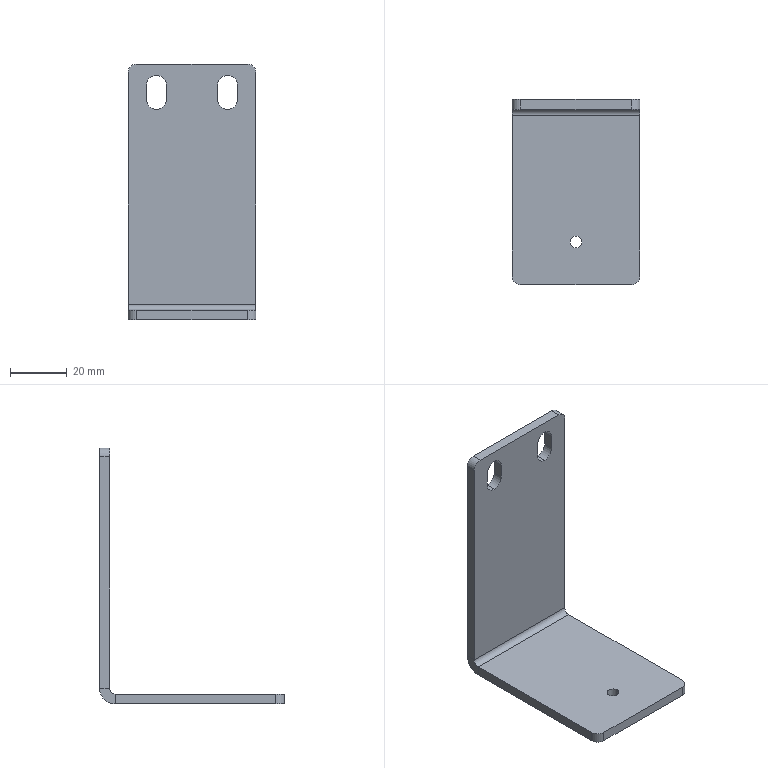Part | SolidWorks | features HoleWzd 2, EdgeFlange 1, Fillet 1, FlatPattern 1, ICE 1, MirrorPattern 1, SMBaseFlange 1, SheetMetal 1 | 1 solid | 30 faces | box 45 x 65 x 90 mm | volume 23018 mm3 | plane 16 | cylinder 14 | commonest cylinder face diameters 7 x6 6 x4 4.2 x2 4 x1 11 x1
STEP:
#1=CARTESIAN_POINT('',(16.,32.5,74.));
#2=VERTEX_POINT('',#1);
#3=CARTESIAN_POINT('',(12.5,32.5,70.5));
#4=VERTEX_POINT('',#3);
#5=CARTESIAN_POINT('',(12.5,32.5,74.));
#6=DIRECTION('',(0.,1.,0.));
#7=DIRECTION('',(0.,0.,-1.));
#8=AXIS2_PLACEMENT_3D('',#5,#6,#7);
#9=CIRCLE('',#8,3.5);
#10=EDGE_CURVE('',#2,#4,#9,.T.);
#11=ORIENTED_EDGE('',*,*,#10,.T.);
#12=CARTESIAN_POINT('',(12.5,29.,70.5));
#13=VERTEX_POINT('',#12);
#14=CARTESIAN_POINT('',(12.5,32.5,70.5));
#15=DIRECTION('',(0.,-1.,0.));
#16=VECTOR('',#15,1000.);
#17=LINE('',#14,#16);
#18=EDGE_CURVE('',#4,#13,#17,.T.);
#19=ORIENTED_EDGE('',*,*,#18,.T.);
#20=CARTESIAN_POINT('',(16.,29.,74.));
#21=VERTEX_POINT('',#20);
#22=CARTESIAN_POINT('',(12.5,29.,74.));
#23=DIRECTION('',(0.,1.,0.));
#24=DIRECTION('',(0.,0.,-1.));
#25=AXIS2_PLACEMENT_3D('',#22,#23,#24);
#26=CIRCLE('',#25,3.5);
#27=EDGE_CURVE('',#21,#13,#26,.T.);
#28=ORIENTED_EDGE('',*,*,#27,.F.);
#29=CARTESIAN_POINT('',(16.,32.5,74.));
#30=DIRECTION('',(0.,-1.,0.));
#31=VECTOR('',#30,1000.);
#32=LINE('',#29,#31);
#33=EDGE_CURVE('',#2,#21,#32,.T.);
#34=ORIENTED_EDGE('',*,*,#33,.F.);
#35=EDGE_LOOP('',(#11,#19,#28,#34));
#36=FACE_OUTER_BOUND('',#35,.T.);
#37=CARTESIAN_POINT('',(12.5,32.5,74.));
#38=DIRECTION('',(0.,-1.,0.));
#39=DIRECTION('',(0.,0.,-1.));
#40=AXIS2_PLACEMENT_3D('',#37,#38,#39);
#41=CYLINDRICAL_SURFACE('',#40,3.5);
#42=ADVANCED_FACE('',(#36),#41,.F.);
#43=CARTESIAN_POINT('',(-12.5,32.5,70.5));
#44=VERTEX_POINT('',#43);
#45=CARTESIAN_POINT('',(-9.,32.5,74.));
#46=VERTEX_POINT('',#45);
#47=CARTESIAN_POINT('',(-12.5,32.5,74.));
#48=DIRECTION('',(0.,-1.,0.));
#49=DIRECTION('',(0.,0.,-1.));
#50=AXIS2_PLACEMENT_3D('',#47,#48,#49);
#51=CIRCLE('',#50,3.5);
#52=EDGE_CURVE('',#44,#46,#51,.T.);
#53=ORIENTED_EDGE('',*,*,#52,.F.);
#54=CARTESIAN_POINT('',(-12.5,29.,70.5));
#55=VERTEX_POINT('',#54);
#56=CARTESIAN_POINT('',(-12.5,32.5,70.5));
#57=DIRECTION('',(0.,-1.,0.));
#58=VECTOR('',#57,1000.);
#59=LINE('',#56,#58);
#60=EDGE_CURVE('',#44,#55,#59,.T.);
#61=ORIENTED_EDGE('',*,*,#60,.T.);
#62=CARTESIAN_POINT('',(-9.,29.,74.));
#63=VERTEX_POINT('',#62);
#64=CARTESIAN_POINT('',(-12.5,29.,74.));
#65=DIRECTION('',(0.,-1.,0.));
#66=DIRECTION('',(0.,0.,-1.));
#67=AXIS2_PLACEMENT_3D('',#64,#65,#66);
#68=CIRCLE('',#67,3.5);
#69=EDGE_CURVE('',#55,#63,#68,.T.);
#70=ORIENTED_EDGE('',*,*,#69,.T.);
#71=CARTESIAN_POINT('',(-9.,32.5,74.));
#72=DIRECTION('',(0.,-1.,0.));
#73=VECTOR('',#72,1000.);
#74=LINE('',#71,#73);
#75=EDGE_CURVE('',#46,#63,#74,.T.);
#76=ORIENTED_EDGE('',*,*,#75,.F.);
#77=EDGE_LOOP('',(#53,#61,#70,#76));
#78=FACE_OUTER_BOUND('',#77,.T.);
#79=CARTESIAN_POINT('',(-12.5,32.5,74.));
#80=DIRECTION('',(0.,-1.,0.));
#81=DIRECTION('',(0.,0.,-1.));
#82=AXIS2_PLACEMENT_3D('',#79,#80,#81);
#83=CYLINDRICAL_SURFACE('',#82,3.5);
#84=ADVANCED_FACE('',(#78),#83,.F.);
#85=CARTESIAN_POINT('',(-2.1,-17.5,-3.5));
#86=VERTEX_POINT('',#85);
#87=CARTESIAN_POINT('',(2.1,-17.5,-3.5));
#88=VERTEX_POINT('',#87);
#89=CARTESIAN_POINT('',(0.,-17.5,-3.5));
#90=DIRECTION('',(0.,0.,1.));
#91=DIRECTION('',(1.,0.,0.));
#92=AXIS2_PLACEMENT_3D('',#89,#90,#91);
#93=CIRCLE('',#92,2.1);
#94=EDGE_CURVE('',#86,#88,#93,.T.);
#95=ORIENTED_EDGE('',*,*,#94,.F.);
#96=CARTESIAN_POINT('',(-2.1,-17.5,0.));
#97=VERTEX_POINT('',#96);
#98=CARTESIAN_POINT('',(-2.1,-17.5,0.));
#99=DIRECTION('',(0.,0.,1.));
#100=VECTOR('',#99,1000.);
#101=LINE('',#98,#100);
#102=EDGE_CURVE('',#86,#97,#101,.T.);
#103=ORIENTED_EDGE('',*,*,#102,.T.);
#104=CARTESIAN_POINT('',(2.1,-17.5,0.));
#105=VERTEX_POINT('',#104);
#106=CARTESIAN_POINT('',(0.,-17.5,0.));
#107=DIRECTION('',(0.,0.,1.));
#108=DIRECTION('',(1.,0.,0.));
#109=AXIS2_PLACEMENT_3D('',#106,#107,#108);
#110=CIRCLE('',#109,2.1);
#111=EDGE_CURVE('',#97,#105,#110,.T.);
#112=ORIENTED_EDGE('',*,*,#111,.T.);
#113=CARTESIAN_POINT('',(2.1,-17.5,0.));
#114=DIRECTION('',(0.,0.,1.));
#115=VECTOR('',#114,1000.);
#116=LINE('',#113,#115);
#117=EDGE_CURVE('',#88,#105,#116,.T.);
#118=ORIENTED_EDGE('',*,*,#117,.F.);
#119=EDGE_LOOP('',(#95,#103,#112,#118));
#120=FACE_OUTER_BOUND('',#119,.T.);
#121=CARTESIAN_POINT('',(0.,-17.5,0.));
#122=DIRECTION('',(0.,0.,1.));
#123=DIRECTION('',(1.,0.,0.));
#124=AXIS2_PLACEMENT_3D('',#121,#122,#123);
#125=CYLINDRICAL_SURFACE('',#124,2.1);
#126=ADVANCED_FACE('',(#120),#125,.F.);
#127=CARTESIAN_POINT('',(-9.,32.5,79.));
#128=VERTEX_POINT('',#127);
#129=CARTESIAN_POINT('',(-16.,32.5,79.));
#130=VERTEX_POINT('',#129);
#131=CARTESIAN_POINT('',(-12.5,32.5,79.));
#132=DIRECTION('',(0.,-1.,0.));
#133=DIRECTION('',(0.,0.,-1.));
#134=AXIS2_PLACEMENT_3D('',#131,#132,#133);
#135=CIRCLE('',#134,3.5);
#136=EDGE_CURVE('',#128,#130,#135,.T.);
#137=ORIENTED_EDGE('',*,*,#136,.T.);
#138=CARTESIAN_POINT('',(-16.,32.5,74.));
#139=VERTEX_POINT('',#138);
#140=CARTESIAN_POINT('',(-16.,32.5,79.));
#141=DIRECTION('',(0.,0.,-1.));
#142=VECTOR('',#141,1000.);
#143=LINE('',#140,#142);
#144=EDGE_CURVE('',#130,#139,#143,.T.);
#145=ORIENTED_EDGE('',*,*,#144,.T.);
#146=CARTESIAN_POINT('',(-12.5,32.5,74.));
#147=DIRECTION('',(0.,-1.,0.));
#148=DIRECTION('',(0.,0.,-1.));
#149=AXIS2_PLACEMENT_3D('',#146,#147,#148);
#150=CIRCLE('',#149,3.5);
#151=EDGE_CURVE('',#139,#44,#150,.T.);
#152=ORIENTED_EDGE('',*,*,#151,.T.);
#153=ORIENTED_EDGE('',*,*,#52,.T.);
#154=CARTESIAN_POINT('',(-9.,32.5,79.));
#155=DIRECTION('',(0.,0.,1.));
#156=VECTOR('',#155,1000.);
#157=LINE('',#154,#156);
#158=EDGE_CURVE('',#46,#128,#157,.T.);
#159=ORIENTED_EDGE('',*,*,#158,.T.);
#160=EDGE_LOOP('',(#137,#145,#152,#153,#159));
#161=FACE_BOUND('',#160,.T.);
#162=CARTESIAN_POINT('',(19.5,32.5,86.5));
#163=VERTEX_POINT('',#162);
#164=CARTESIAN_POINT('',(-19.5,32.5,86.5));
#165=VERTEX_POINT('',#164);
#166=CARTESIAN_POINT('',(-22.5,32.5,86.5));
#167=DIRECTION('',(-1.,0.,0.));
#168=VECTOR('',#167,1000.);
#169=LINE('',#166,#168);
#170=EDGE_CURVE('',#163,#165,#169,.T.);
#171=ORIENTED_EDGE('',*,*,#170,.F.);
#172=CARTESIAN_POINT('',(22.5,32.5,83.5));
#173=VERTEX_POINT('',#172);
#174=CARTESIAN_POINT('',(19.5,32.5,83.5));
#175=DIRECTION('',(0.,1.,0.));
#176=DIRECTION('',(0.,0.,1.));
#177=AXIS2_PLACEMENT_3D('',#174,#175,#176);
#178=CIRCLE('',#177,3.);
#179=EDGE_CURVE('',#163,#173,#178,.T.);
#180=ORIENTED_EDGE('',*,*,#179,.T.);
#181=CARTESIAN_POINT('',(22.5,32.5,2.));
#182=VERTEX_POINT('',#181);
#183=CARTESIAN_POINT('',(22.5,32.5,86.5));
#184=DIRECTION('',(0.,0.,1.));
#185=VECTOR('',#184,1000.);
#186=LINE('',#183,#185);
#187=EDGE_CURVE('',#182,#173,#186,.T.);
#188=ORIENTED_EDGE('',*,*,#187,.F.);
#189=CARTESIAN_POINT('',(-22.5,32.5,2.));
#190=VERTEX_POINT('',#189);
#191=CARTESIAN_POINT('',(0.,32.5,2.));
#192=DIRECTION('',(-1.,0.,0.));
#193=VECTOR('',#192,1000.);
#194=LINE('',#191,#193);
#195=EDGE_CURVE('',#182,#190,#194,.T.);
#196=ORIENTED_EDGE('',*,*,#195,.T.);
#197=CARTESIAN_POINT('',(-22.5,32.5,83.5));
#198=VERTEX_POINT('',#197);
#199=CARTESIAN_POINT('',(-22.5,32.5,0.));
#200=DIRECTION('',(0.,0.,-1.));
#201=VECTOR('',#200,1000.);
#202=LINE('',#199,#201);
#203=EDGE_CURVE('',#198,#190,#202,.T.);
#204=ORIENTED_EDGE('',*,*,#203,.F.);
#205=CARTESIAN_POINT('',(-19.5,32.5,83.5));
#206=DIRECTION('',(0.,1.,0.));
#207=DIRECTION('',(0.,0.,1.));
#208=AXIS2_PLACEMENT_3D('',#205,#206,#207);
#209=CIRCLE('',#208,3.);
#210=EDGE_CURVE('',#198,#165,#209,.T.);
#211=ORIENTED_EDGE('',*,*,#210,.T.);
#212=EDGE_LOOP('',(#171,#180,#188,#196,#204,#211));
#213=FACE_OUTER_BOUND('',#212,.T.);
#214=ORIENTED_EDGE('',*,*,#10,.F.);
#215=CARTESIAN_POINT('',(16.,32.5,79.));
#216=VERTEX_POINT('',#215);
#217=CARTESIAN_POINT('',(16.,32.5,79.));
#218=DIRECTION('',(0.,0.,-1.));
#219=VECTOR('',#218,1000.);
#220=LINE('',#217,#219);
#221=EDGE_CURVE('',#216,#2,#220,.T.);
#222=ORIENTED_EDGE('',*,*,#221,.F.);
#223=CARTESIAN_POINT('',(9.,32.5,79.));
#224=VERTEX_POINT('',#223);
#225=CARTESIAN_POINT('',(12.5,32.5,79.));
#226=DIRECTION('',(0.,1.,0.));
#227=DIRECTION('',(0.,0.,-1.));
#228=AXIS2_PLACEMENT_3D('',#225,#226,#227);
#229=CIRCLE('',#228,3.5);
#230=EDGE_CURVE('',#224,#216,#229,.T.);
#231=ORIENTED_EDGE('',*,*,#230,.F.);
#232=CARTESIAN_POINT('',(9.,32.5,74.));
#233=VERTEX_POINT('',#232);
#234=CARTESIAN_POINT('',(9.,32.5,79.));
#235=DIRECTION('',(0.,0.,1.));
#236=VECTOR('',#235,1000.);
#237=LINE('',#234,#236);
#238=EDGE_CURVE('',#233,#224,#237,.T.);
#239=ORIENTED_EDGE('',*,*,#238,.F.);
#240=CARTESIAN_POINT('',(12.5,32.5,74.));
#241=DIRECTION('',(0.,1.,0.));
#242=DIRECTION('',(0.,0.,-1.));
#243=AXIS2_PLACEMENT_3D('',#240,#241,#242);
#244=CIRCLE('',#243,3.5);
#245=EDGE_CURVE('',#4,#233,#244,.T.);
#246=ORIENTED_EDGE('',*,*,#245,.F.);
#247=EDGE_LOOP('',(#214,#222,#231,#239,#246));
#248=FACE_BOUND('',#247,.T.);
#249=CARTESIAN_POINT('',(0.,32.5,0.));
#250=DIRECTION('',(0.,1.,0.));
#251=DIRECTION('',(0.,0.,1.));
#252=AXIS2_PLACEMENT_3D('',#249,#250,#251);
#253=PLANE('',#252);
#254=ADVANCED_FACE('',(#161,#213,#248),#253,.T.);
#255=CARTESIAN_POINT('',(-16.,29.,79.));
#256=VERTEX_POINT('',#255);
#257=CARTESIAN_POINT('',(-16.,29.,74.));
#258=VERTEX_POINT('',#257);
#259=CARTESIAN_POINT('',(-16.,29.,79.));
#260=DIRECTION('',(0.,0.,-1.));
#261=VECTOR('',#260,1000.);
#262=LINE('',#259,#261);
#263=EDGE_CURVE('',#256,#258,#262,.T.);
#264=ORIENTED_EDGE('',*,*,#263,.F.);
#265=CARTESIAN_POINT('',(-9.,29.,79.));
#266=VERTEX_POINT('',#265);
#267=CARTESIAN_POINT('',(-12.5,29.,79.));
#268=DIRECTION('',(0.,-1.,0.));
#269=DIRECTION('',(0.,0.,-1.));
#270=AXIS2_PLACEMENT_3D('',#267,#268,#269);
#271=CIRCLE('',#270,3.5);
#272=EDGE_CURVE('',#266,#256,#271,.T.);
#273=ORIENTED_EDGE('',*,*,#272,.F.);
#274=CARTESIAN_POINT('',(-9.,29.,79.));
#275=DIRECTION('',(0.,0.,1.));
#276=VECTOR('',#275,1000.);
#277=LINE('',#274,#276);
#278=EDGE_CURVE('',#63,#266,#277,.T.);
#279=ORIENTED_EDGE('',*,*,#278,.F.);
#280=ORIENTED_EDGE('',*,*,#69,.F.);
#281=CARTESIAN_POINT('',(-12.5,29.,74.));
#282=DIRECTION('',(0.,-1.,0.));
#283=DIRECTION('',(0.,0.,-1.));
#284=AXIS2_PLACEMENT_3D('',#281,#282,#283);
#285=CIRCLE('',#284,3.5);
#286=EDGE_CURVE('',#258,#55,#285,.T.);
#287=ORIENTED_EDGE('',*,*,#286,.F.);
#288=EDGE_LOOP('',(#264,#273,#279,#280,#287));
#289=FACE_BOUND('',#288,.T.);
#290=CARTESIAN_POINT('',(22.5,29.,2.));
#291=VERTEX_POINT('',#290);
#292=CARTESIAN_POINT('',(22.5,29.,83.5));
#293=VERTEX_POINT('',#292);
#294=CARTESIAN_POINT('',(22.5,29.,0.));
#295=DIRECTION('',(0.,0.,1.));
#296=VECTOR('',#295,1000.);
#297=LINE('',#294,#296);
#298=EDGE_CURVE('',#291,#293,#297,.T.);
#299=ORIENTED_EDGE('',*,*,#298,.T.);
#300=CARTESIAN_POINT('',(19.5,29.,86.5));
#301=VERTEX_POINT('',#300);
#302=CARTESIAN_POINT('',(19.5,29.,83.5));
#303=DIRECTION('',(0.,-1.,0.));
#304=DIRECTION('',(0.,0.,1.));
#305=AXIS2_PLACEMENT_3D('',#302,#303,#304);
#306=CIRCLE('',#305,3.);
#307=EDGE_CURVE('',#293,#301,#306,.T.);
#308=ORIENTED_EDGE('',*,*,#307,.T.);
#309=CARTESIAN_POINT('',(-19.5,29.,86.5));
#310=VERTEX_POINT('',#309);
#311=CARTESIAN_POINT('',(0.,29.,86.5));
#312=DIRECTION('',(-1.,0.,0.));
#313=VECTOR('',#312,1000.);
#314=LINE('',#311,#313);
#315=EDGE_CURVE('',#301,#310,#314,.T.);
#316=ORIENTED_EDGE('',*,*,#315,.T.);
#317=CARTESIAN_POINT('',(-22.5,29.,83.5));
#318=VERTEX_POINT('',#317);
#319=CARTESIAN_POINT('',(-19.5,29.,83.5));
#320=DIRECTION('',(0.,-1.,0.));
#321=DIRECTION('',(0.,0.,1.));
#322=AXIS2_PLACEMENT_3D('',#319,#320,#321);
#323=CIRCLE('',#322,3.);
#324=EDGE_CURVE('',#310,#318,#323,.T.);
#325=ORIENTED_EDGE('',*,*,#324,.T.);
#326=CARTESIAN_POINT('',(-22.5,29.,2.));
#327=VERTEX_POINT('',#326);
#328=CARTESIAN_POINT('',(-22.5,29.,0.));
#329=DIRECTION('',(0.,0.,-1.));
#330=VECTOR('',#329,1000.);
#331=LINE('',#328,#330);
#332=EDGE_CURVE('',#318,#327,#331,.T.);
#333=ORIENTED_EDGE('',*,*,#332,.T.);
#334=CARTESIAN_POINT('',(22.5,29.,2.));
#335=DIRECTION('',(-1.,0.,0.));
#336=VECTOR('',#335,1000.);
#337=LINE('',#334,#336);
#338=EDGE_CURVE('',#291,#327,#337,.T.);
#339=ORIENTED_EDGE('',*,*,#338,.F.);
#340=EDGE_LOOP('',(#299,#308,#316,#325,#333,#339));
#341=FACE_OUTER_BOUND('',#340,.T.);
#342=CARTESIAN_POINT('',(9.,29.,79.));
#343=VERTEX_POINT('',#342);
#344=CARTESIAN_POINT('',(16.,29.,79.));
#345=VERTEX_POINT('',#344);
#346=CARTESIAN_POINT('',(12.5,29.,79.));
#347=DIRECTION('',(0.,1.,0.));
#348=DIRECTION('',(0.,0.,-1.));
#349=AXIS2_PLACEMENT_3D('',#346,#347,#348);
#350=CIRCLE('',#349,3.5);
#351=EDGE_CURVE('',#343,#345,#350,.T.);
#352=ORIENTED_EDGE('',*,*,#351,.T.);
#353=CARTESIAN_POINT('',(16.,29.,79.));
#354=DIRECTION('',(0.,0.,-1.));
#355=VECTOR('',#354,1000.);
#356=LINE('',#353,#355);
#357=EDGE_CURVE('',#345,#21,#356,.T.);
#358=ORIENTED_EDGE('',*,*,#357,.T.);
#359=ORIENTED_EDGE('',*,*,#27,.T.);
#360=CARTESIAN_POINT('',(9.,29.,74.));
#361=VERTEX_POINT('',#360);
#362=CARTESIAN_POINT('',(12.5,29.,74.));
#363=DIRECTION('',(0.,1.,0.));
#364=DIRECTION('',(0.,0.,-1.));
#365=AXIS2_PLACEMENT_3D('',#362,#363,#364);
#366=CIRCLE('',#365,3.5);
#367=EDGE_CURVE('',#13,#361,#366,.T.);
#368=ORIENTED_EDGE('',*,*,#367,.T.);
#369=CARTESIAN_POINT('',(9.,29.,79.));
#370=DIRECTION('',(0.,0.,1.));
#371=VECTOR('',#370,1000.);
#372=LINE('',#369,#371);
#373=EDGE_CURVE('',#361,#343,#372,.T.);
#374=ORIENTED_EDGE('',*,*,#373,.T.);
#375=EDGE_LOOP('',(#352,#358,#359,#368,#374));
#376=FACE_BOUND('',#375,.T.);
#377=CARTESIAN_POINT('',(0.,29.,0.));
#378=DIRECTION('',(0.,1.,0.));
#379=DIRECTION('',(0.,0.,1.));
#380=AXIS2_PLACEMENT_3D('',#377,#378,#379);
#381=PLANE('',#380);
#382=ADVANCED_FACE('',(#289,#341,#376),#381,.F.);
#383=CARTESIAN_POINT('',(-22.5,27.,-3.5));
#384=VERTEX_POINT('',#383);
#385=CARTESIAN_POINT('',(-22.5,-29.5,-3.5));
#386=VERTEX_POINT('',#385);
#387=CARTESIAN_POINT('',(-22.5,32.5,-3.5));
#388=DIRECTION('',(0.,-1.,0.));
#389=VECTOR('',#388,1000.);
#390=LINE('',#387,#389);
#391=EDGE_CURVE('',#384,#386,#390,.T.);
#392=ORIENTED_EDGE('',*,*,#391,.T.);
#393=CARTESIAN_POINT('',(-22.5,-29.5,0.));
#394=VERTEX_POINT('',#393);
#395=CARTESIAN_POINT('',(-22.5,-29.5,-3.5));
#396=DIRECTION('',(0.,0.,1.));
#397=VECTOR('',#396,1000.);
#398=LINE('',#395,#397);
#399=EDGE_CURVE('',#386,#394,#398,.T.);
#400=ORIENTED_EDGE('',*,*,#399,.T.);
#401=CARTESIAN_POINT('',(-22.5,27.,0.));
#402=VERTEX_POINT('',#401);
#403=CARTESIAN_POINT('',(-22.5,32.5,0.));
#404=DIRECTION('',(0.,-1.,0.));
#405=VECTOR('',#404,1000.);
#406=LINE('',#403,#405);
#407=EDGE_CURVE('',#402,#394,#406,.T.);
#408=ORIENTED_EDGE('',*,*,#407,.F.);
#409=CARTESIAN_POINT('',(-22.5,27.,0.));
#410=DIRECTION('',(0.,0.,-1.));
#411=VECTOR('',#410,1000.);
#412=LINE('',#409,#411);
#413=EDGE_CURVE('',#402,#384,#412,.T.);
#414=ORIENTED_EDGE('',*,*,#413,.T.);
#415=EDGE_LOOP('',(#392,#400,#408,#414));
#416=FACE_OUTER_BOUND('',#415,.T.);
#417=CARTESIAN_POINT('',(-22.5,32.5,-3.5));
#418=DIRECTION('',(-1.,0.,0.));
#419=DIRECTION('',(0.,-1.,0.));
#420=AXIS2_PLACEMENT_3D('',#417,#418,#419);
#421=PLANE('',#420);
#422=ADVANCED_FACE('',(#416),#421,.T.);
#423=CARTESIAN_POINT('',(0.,-17.5,-3.5));
#424=DIRECTION('',(0.,0.,1.));
#425=DIRECTION('',(1.,0.,0.));
#426=AXIS2_PLACEMENT_3D('',#423,#424,#425);
#427=CIRCLE('',#426,2.1);
#428=EDGE_CURVE('',#88,#86,#427,.T.);
#429=ORIENTED_EDGE('',*,*,#428,.T.);
#430=ORIENTED_EDGE('',*,*,#94,.T.);
#431=EDGE_LOOP('',(#429,#430));
#432=FACE_BOUND('',#431,.T.);
#433=CARTESIAN_POINT('',(22.5,-29.5,-3.5));
#434=VERTEX_POINT('',#433);
#435=CARTESIAN_POINT('',(22.5,27.,-3.5));
#436=VERTEX_POINT('',#435);
#437=CARTESIAN_POINT('',(22.5,32.5,-3.5));
#438=DIRECTION('',(0.,1.,0.));
#439=VECTOR('',#438,1000.);
#440=LINE('',#437,#439);
#441=EDGE_CURVE('',#434,#436,#440,.T.);
#442=ORIENTED_EDGE('',*,*,#441,.F.);
#443=CARTESIAN_POINT('',(19.5,-32.5,-3.5));
#444=VERTEX_POINT('',#443);
#445=CARTESIAN_POINT('',(19.5,-29.5,-3.5));
#446=DIRECTION('',(0.,0.,-1.));
#447=DIRECTION('',(1.,0.,0.));
#448=AXIS2_PLACEMENT_3D('',#445,#446,#447);
#449=CIRCLE('',#448,3.);
#450=EDGE_CURVE('',#434,#444,#449,.T.);
#451=ORIENTED_EDGE('',*,*,#450,.T.);
#452=CARTESIAN_POINT('',(-19.5,-32.5,-3.5));
#453=VERTEX_POINT('',#452);
#454=CARTESIAN_POINT('',(-22.5,-32.5,-3.5));
#455=DIRECTION('',(1.,0.,0.));
#456=VECTOR('',#455,1000.);
#457=LINE('',#454,#456);
#458=EDGE_CURVE('',#453,#444,#457,.T.);
#459=ORIENTED_EDGE('',*,*,#458,.F.);
#460=CARTESIAN_POINT('',(-19.5,-29.5,-3.5));
#461=DIRECTION('',(0.,0.,-1.));
#462=DIRECTION('',(1.,0.,0.));
#463=AXIS2_PLACEMENT_3D('',#460,#461,#462);
#464=CIRCLE('',#463,3.);
#465=EDGE_CURVE('',#453,#386,#464,.T.);
#466=ORIENTED_EDGE('',*,*,#465,.T.);
#467=ORIENTED_EDGE('',*,*,#391,.F.);
#468=CARTESIAN_POINT('',(-22.5,27.,-3.5));
#469=DIRECTION('',(1.,0.,0.));
#470=VECTOR('',#469,1000.);
#471=LINE('',#468,#470);
#472=EDGE_CURVE('',#384,#436,#471,.T.);
#473=ORIENTED_EDGE('',*,*,#472,.T.);
#474=EDGE_LOOP('',(#442,#451,#459,#466,#467,#473));
#475=FACE_OUTER_BOUND('',#474,.T.);
#476=CARTESIAN_POINT('',(0.,0.,-3.5));
#477=DIRECTION('',(0.,0.,1.));
#478=DIRECTION('',(1.,0.,0.));
#479=AXIS2_PLACEMENT_3D('',#476,#477,#478);
#480=PLANE('',#479);
#481=ADVANCED_FACE('',(#432,#475),#480,.F.);
#482=CARTESIAN_POINT('',(0.,-17.5,0.));
#483=DIRECTION('',(0.,0.,1.));
#484=DIRECTION('',(1.,0.,0.));
#485=AXIS2_PLACEMENT_3D('',#482,#483,#484);
#486=CIRCLE('',#485,2.1);
#487=EDGE_CURVE('',#105,#97,#486,.T.);
#488=ORIENTED_EDGE('',*,*,#487,.F.);
#489=ORIENTED_EDGE('',*,*,#111,.F.);
#490=EDGE_LOOP('',(#488,#489));
#491=FACE_BOUND('',#490,.T.);
#492=CARTESIAN_POINT('',(-19.5,-32.5,0.));
#493=VERTEX_POINT('',#492);
#494=CARTESIAN_POINT('',(19.5,-32.5,0.));
#495=VERTEX_POINT('',#494);
#496=CARTESIAN_POINT('',(-22.5,-32.5,0.));
#497=DIRECTION('',(1.,0.,0.));
#498=VECTOR('',#497,1000.);
#499=LINE('',#496,#498);
#500=EDGE_CURVE('',#493,#495,#499,.T.);
#501=ORIENTED_EDGE('',*,*,#500,.T.);
#502=CARTESIAN_POINT('',(22.5,-29.5,0.));
#503=VERTEX_POINT('',#502);
#504=CARTESIAN_POINT('',(19.5,-29.5,0.));
#505=DIRECTION('',(0.,0.,1.));
#506=DIRECTION('',(1.,0.,0.));
#507=AXIS2_PLACEMENT_3D('',#504,#505,#506);
#508=CIRCLE('',#507,3.);
#509=EDGE_CURVE('',#495,#503,#508,.T.);
#510=ORIENTED_EDGE('',*,*,#509,.T.);
#511=CARTESIAN_POINT('',(22.5,27.,0.));
#512=VERTEX_POINT('',#511);
#513=CARTESIAN_POINT('',(22.5,32.5,0.));
#514=DIRECTION('',(0.,1.,0.));
#515=VECTOR('',#514,1000.);
#516=LINE('',#513,#515);
#517=EDGE_CURVE('',#503,#512,#516,.T.);
#518=ORIENTED_EDGE('',*,*,#517,.T.);
#519=CARTESIAN_POINT('',(-22.5,27.,0.));
#520=DIRECTION('',(1.,0.,0.));
#521=VECTOR('',#520,1000.);
#522=LINE('',#519,#521);
#523=EDGE_CURVE('',#402,#512,#522,.T.);
#524=ORIENTED_EDGE('',*,*,#523,.F.);
#525=ORIENTED_EDGE('',*,*,#407,.T.);
#526=CARTESIAN_POINT('',(-19.5,-29.5,0.));
#527=DIRECTION('',(0.,0.,1.));
#528=DIRECTION('',(1.,0.,0.));
#529=AXIS2_PLACEMENT_3D('',#526,#527,#528);
#530=CIRCLE('',#529,3.);
#531=EDGE_CURVE('',#394,#493,#530,.T.);
#532=ORIENTED_EDGE('',*,*,#531,.T.);
#533=EDGE_LOOP('',(#501,#510,#518,#524,#525,#532));
#534=FACE_OUTER_BOUND('',#533,.T.);
#535=CARTESIAN_POINT('',(0.,0.,0.));
#536=DIRECTION('',(0.,0.,1.));
#537=DIRECTION('',(1.,0.,0.));
#538=AXIS2_PLACEMENT_3D('',#535,#536,#537);
#539=PLANE('',#538);
#540=ADVANCED_FACE('',(#491,#534),#539,.T.);
#541=ORIENTED_EDGE('',*,*,#517,.F.);
#542=CARTESIAN_POINT('',(22.5,-29.5,-3.5));
#543=DIRECTION('',(0.,0.,-1.));
#544=VECTOR('',#543,1000.);
#545=LINE('',#542,#544);
#546=EDGE_CURVE('',#503,#434,#545,.T.);
#547=ORIENTED_EDGE('',*,*,#546,.T.);
#548=ORIENTED_EDGE('',*,*,#441,.T.);
#549=CARTESIAN_POINT('',(22.5,27.,0.));
#550=DIRECTION('',(0.,0.,-1.));
#551=VECTOR('',#550,1000.);
#552=LINE('',#549,#551);
#553=EDGE_CURVE('',#512,#436,#552,.T.);
#554=ORIENTED_EDGE('',*,*,#553,.F.);
#555=EDGE_LOOP('',(#541,#547,#548,#554));
#556=FACE_OUTER_BOUND('',#555,.T.);
#557=CARTESIAN_POINT('',(22.5,32.5,-3.5));
#558=DIRECTION('',(1.,0.,0.));
#559=DIRECTION('',(0.,1.,0.));
#560=AXIS2_PLACEMENT_3D('',#557,#558,#559);
#561=PLANE('',#560);
#562=ADVANCED_FACE('',(#556),#561,.T.);
#563=ORIENTED_EDGE('',*,*,#458,.T.);
#564=CARTESIAN_POINT('',(19.5,-32.5,-3.5));
#565=DIRECTION('',(0.,0.,1.));
#566=VECTOR('',#565,1000.);
#567=LINE('',#564,#566);
#568=EDGE_CURVE('',#444,#495,#567,.T.);
#569=ORIENTED_EDGE('',*,*,#568,.T.);
#570=ORIENTED_EDGE('',*,*,#500,.F.);
#571=CARTESIAN_POINT('',(-19.5,-32.5,-3.5));
#572=DIRECTION('',(0.,0.,-1.));
#573=VECTOR('',#572,1000.);
#574=LINE('',#571,#573);
#575=EDGE_CURVE('',#493,#453,#574,.T.);
#576=ORIENTED_EDGE('',*,*,#575,.T.);
#577=EDGE_LOOP('',(#563,#569,#570,#576));
#578=FACE_OUTER_BOUND('',#577,.T.);
#579=CARTESIAN_POINT('',(-22.5,-32.5,-3.5));
#580=DIRECTION('',(0.,-1.,0.));
#581=DIRECTION('',(0.,0.,-1.));
#582=AXIS2_PLACEMENT_3D('',#579,#580,#581);
#583=PLANE('',#582);
#584=ADVANCED_FACE('',(#578),#583,.T.);
#585=CARTESIAN_POINT('',(22.5,32.5,2.));
#586=DIRECTION('',(0.,1.,0.));
#587=VECTOR('',#586,1000.);
#588=LINE('',#585,#587);
#589=EDGE_CURVE('',#291,#182,#588,.T.);
#590=ORIENTED_EDGE('',*,*,#589,.F.);
#591=CARTESIAN_POINT('',(22.5,27.,2.));
#592=DIRECTION('',(1.,0.,0.));
#593=DIRECTION('',(0.,0.,1.));
#594=AXIS2_PLACEMENT_3D('',#591,#592,#593);
#595=CIRCLE('',#594,2.);
#596=EDGE_CURVE('',#512,#291,#595,.T.);
#597=ORIENTED_EDGE('',*,*,#596,.F.);
#598=ORIENTED_EDGE('',*,*,#553,.T.);
#599=CARTESIAN_POINT('',(22.5,27.,2.));
#600=DIRECTION('',(1.,0.,0.));
#601=DIRECTION('',(0.,0.,1.));
#602=AXIS2_PLACEMENT_3D('',#599,#600,#601);
#603=CIRCLE('',#602,5.5);
#604=EDGE_CURVE('',#436,#182,#603,.T.);
#605=ORIENTED_EDGE('',*,*,#604,.T.);
#606=EDGE_LOOP('',(#590,#597,#598,#605));
#607=FACE_OUTER_BOUND('',#606,.T.);
#608=CARTESIAN_POINT('',(22.5,27.,2.));
#609=DIRECTION('',(1.,0.,0.));
#610=DIRECTION('',(0.,0.,-1.));
#611=AXIS2_PLACEMENT_3D('',#608,#609,#610);
#612=PLANE('',#611);
#613=ADVANCED_FACE('',(#607),#612,.T.);
#614=CARTESIAN_POINT('',(-22.5,27.,2.));
#615=DIRECTION('',(-1.,0.,0.));
#616=DIRECTION('',(0.,0.,1.));
#617=AXIS2_PLACEMENT_3D('',#614,#615,#616);
#618=CIRCLE('',#617,2.);
#619=EDGE_CURVE('',#327,#402,#618,.T.);
#620=ORIENTED_EDGE('',*,*,#619,.F.);
#621=CARTESIAN_POINT('',(-22.5,29.,2.));
#622=DIRECTION('',(0.,1.,0.));
#623=VECTOR('',#622,1000.);
#624=LINE('',#621,#623);
#625=EDGE_CURVE('',#327,#190,#624,.T.);
#626=ORIENTED_EDGE('',*,*,#625,.T.);
#627=CARTESIAN_POINT('',(-22.5,27.,2.));
#628=DIRECTION('',(-1.,0.,0.));
#629=DIRECTION('',(0.,0.,1.));
#630=AXIS2_PLACEMENT_3D('',#627,#628,#629);
#631=CIRCLE('',#630,5.5);
#632=EDGE_CURVE('',#190,#384,#631,.T.);
#633=ORIENTED_EDGE('',*,*,#632,.T.);
#634=ORIENTED_EDGE('',*,*,#413,.F.);
#635=EDGE_LOOP('',(#620,#626,#633,#634));
#636=FACE_OUTER_BOUND('',#635,.T.);
#637=CARTESIAN_POINT('',(-22.5,27.,2.));
#638=DIRECTION('',(1.,0.,0.));
#639=DIRECTION('',(0.,0.,-1.));
#640=AXIS2_PLACEMENT_3D('',#637,#638,#639);
#641=PLANE('',#640);
#642=ADVANCED_FACE('',(#636),#641,.F.);
#643=ORIENTED_EDGE('',*,*,#472,.F.);
#644=ORIENTED_EDGE('',*,*,#632,.F.);
#645=ORIENTED_EDGE('',*,*,#195,.F.);
#646=ORIENTED_EDGE('',*,*,#604,.F.);
#647=EDGE_LOOP('',(#643,#644,#645,#646));
#648=FACE_OUTER_BOUND('',#647,.T.);
#649=CARTESIAN_POINT('',(-22.5,27.,2.));
#650=DIRECTION('',(-1.,0.,0.));
#651=DIRECTION('',(0.,1.,0.));
#652=AXIS2_PLACEMENT_3D('',#649,#650,#651);
#653=CYLINDRICAL_SURFACE('',#652,5.5);
#654=ADVANCED_FACE('',(#648),#653,.T.);
#655=ORIENTED_EDGE('',*,*,#523,.T.);
#656=ORIENTED_EDGE('',*,*,#596,.T.);
#657=ORIENTED_EDGE('',*,*,#338,.T.);
#658=ORIENTED_EDGE('',*,*,#619,.T.);
#659=EDGE_LOOP('',(#655,#656,#657,#658));
#660=FACE_OUTER_BOUND('',#659,.T.);
#661=CARTESIAN_POINT('',(-22.5,27.,2.));
#662=DIRECTION('',(-1.,0.,0.));
#663=DIRECTION('',(0.,1.,0.));
#664=AXIS2_PLACEMENT_3D('',#661,#662,#663);
#665=CYLINDRICAL_SURFACE('',#664,2.);
#666=ADVANCED_FACE('',(#660),#665,.F.);
#667=ORIENTED_EDGE('',*,*,#332,.F.);
#668=CARTESIAN_POINT('',(-22.5,32.5,83.5));
#669=DIRECTION('',(0.,1.,0.));
#670=VECTOR('',#669,1000.);
#671=LINE('',#668,#670);
#672=EDGE_CURVE('',#318,#198,#671,.T.);
#673=ORIENTED_EDGE('',*,*,#672,.T.);
#674=ORIENTED_EDGE('',*,*,#203,.T.);
#675=ORIENTED_EDGE('',*,*,#625,.F.);
#676=EDGE_LOOP('',(#667,#673,#674,#675));
#677=FACE_OUTER_BOUND('',#676,.T.);
#678=CARTESIAN_POINT('',(-22.5,32.5,0.));
#679=DIRECTION('',(-1.,0.,0.));
#680=DIRECTION('',(0.,0.,1.));
#681=AXIS2_PLACEMENT_3D('',#678,#679,#680);
#682=PLANE('',#681);
#683=ADVANCED_FACE('',(#677),#682,.T.);
#684=ORIENTED_EDGE('',*,*,#187,.T.);
#685=CARTESIAN_POINT('',(22.5,32.5,83.5));
#686=DIRECTION('',(0.,-1.,0.));
#687=VECTOR('',#686,1000.);
#688=LINE('',#685,#687);
#689=EDGE_CURVE('',#173,#293,#688,.T.);
#690=ORIENTED_EDGE('',*,*,#689,.T.);
#691=ORIENTED_EDGE('',*,*,#298,.F.);
#692=ORIENTED_EDGE('',*,*,#589,.T.);
#693=EDGE_LOOP('',(#684,#690,#691,#692));
#694=FACE_OUTER_BOUND('',#693,.T.);
#695=CARTESIAN_POINT('',(22.5,32.5,86.5));
#696=DIRECTION('',(1.,0.,0.));
#697=DIRECTION('',(0.,0.,-1.));
#698=AXIS2_PLACEMENT_3D('',#695,#696,#697);
#699=PLANE('',#698);
#700=ADVANCED_FACE('',(#694),#699,.T.);
#701=ORIENTED_EDGE('',*,*,#315,.F.);
#702=CARTESIAN_POINT('',(19.5,32.5,86.5));
#703=DIRECTION('',(0.,1.,0.));
#704=VECTOR('',#703,1000.);
#705=LINE('',#702,#704);
#706=EDGE_CURVE('',#301,#163,#705,.T.);
#707=ORIENTED_EDGE('',*,*,#706,.T.);
#708=ORIENTED_EDGE('',*,*,#170,.T.);
#709=CARTESIAN_POINT('',(-19.5,32.5,86.5));
#710=DIRECTION('',(0.,-1.,0.));
#711=VECTOR('',#710,1000.);
#712=LINE('',#709,#711);
#713=EDGE_CURVE('',#165,#310,#712,.T.);
#714=ORIENTED_EDGE('',*,*,#713,.T.);
#715=EDGE_LOOP('',(#701,#707,#708,#714));
#716=FACE_OUTER_BOUND('',#715,.T.);
#717=CARTESIAN_POINT('',(-22.5,32.5,86.5));
#718=DIRECTION('',(0.,0.,1.));
#719=DIRECTION('',(0.,-1.,0.));
#720=AXIS2_PLACEMENT_3D('',#717,#718,#719);
#721=PLANE('',#720);
#722=ADVANCED_FACE('',(#716),#721,.T.);
#723=ORIENTED_EDGE('',*,*,#102,.F.);
#724=ORIENTED_EDGE('',*,*,#428,.F.);
#725=ORIENTED_EDGE('',*,*,#117,.T.);
#726=ORIENTED_EDGE('',*,*,#487,.T.);
#727=EDGE_LOOP('',(#723,#724,#725,#726));
#728=FACE_OUTER_BOUND('',#727,.T.);
#729=CARTESIAN_POINT('',(0.,-17.5,0.));
#730=DIRECTION('',(0.,0.,1.));
#731=DIRECTION('',(1.,0.,0.));
#732=AXIS2_PLACEMENT_3D('',#729,#730,#731);
#733=CYLINDRICAL_SURFACE('',#732,2.1);
#734=ADVANCED_FACE('',(#728),#733,.F.);
#735=ORIENTED_EDGE('',*,*,#450,.F.);
#736=ORIENTED_EDGE('',*,*,#546,.F.);
#737=ORIENTED_EDGE('',*,*,#509,.F.);
#738=ORIENTED_EDGE('',*,*,#568,.F.);
#739=EDGE_LOOP('',(#735,#736,#737,#738));
#740=FACE_OUTER_BOUND('',#739,.T.);
#741=CARTESIAN_POINT('',(19.5,-29.5,-3.5));
#742=DIRECTION('',(0.,0.,1.));
#743=DIRECTION('',(1.,0.,0.));
#744=AXIS2_PLACEMENT_3D('',#741,#742,#743);
#745=CYLINDRICAL_SURFACE('',#744,3.);
#746=ADVANCED_FACE('',(#740),#745,.T.);
#747=ORIENTED_EDGE('',*,*,#465,.F.);
#748=ORIENTED_EDGE('',*,*,#575,.F.);
#749=ORIENTED_EDGE('',*,*,#531,.F.);
#750=ORIENTED_EDGE('',*,*,#399,.F.);
#751=EDGE_LOOP('',(#747,#748,#749,#750));
#752=FACE_OUTER_BOUND('',#751,.T.);
#753=CARTESIAN_POINT('',(-19.5,-29.5,-3.5));
#754=DIRECTION('',(0.,0.,1.));
#755=DIRECTION('',(1.,0.,0.));
#756=AXIS2_PLACEMENT_3D('',#753,#754,#755);
#757=CYLINDRICAL_SURFACE('',#756,3.);
#758=ADVANCED_FACE('',(#752),#757,.T.);
#759=ORIENTED_EDGE('',*,*,#179,.F.);
#760=ORIENTED_EDGE('',*,*,#706,.F.);
#761=ORIENTED_EDGE('',*,*,#307,.F.);
#762=ORIENTED_EDGE('',*,*,#689,.F.);
#763=EDGE_LOOP('',(#759,#760,#761,#762));
#764=FACE_OUTER_BOUND('',#763,.T.);
#765=CARTESIAN_POINT('',(19.5,32.5,83.5));
#766=DIRECTION('',(0.,-1.,0.));
#767=DIRECTION('',(0.,0.,-1.));
#768=AXIS2_PLACEMENT_3D('',#765,#766,#767);
#769=CYLINDRICAL_SURFACE('',#768,3.);
#770=ADVANCED_FACE('',(#764),#769,.T.);
#771=ORIENTED_EDGE('',*,*,#210,.F.);
#772=ORIENTED_EDGE('',*,*,#672,.F.);
#773=ORIENTED_EDGE('',*,*,#324,.F.);
#774=ORIENTED_EDGE('',*,*,#713,.F.);
#775=EDGE_LOOP('',(#771,#772,#773,#774));
#776=FACE_OUTER_BOUND('',#775,.T.);
#777=CARTESIAN_POINT('',(-19.5,32.5,83.5));
#778=DIRECTION('',(0.,-1.,0.));
#779=DIRECTION('',(0.,0.,-1.));
#780=AXIS2_PLACEMENT_3D('',#777,#778,#779);
#781=CYLINDRICAL_SURFACE('',#780,3.);
#782=ADVANCED_FACE('',(#776),#781,.T.);
#783=ORIENTED_EDGE('',*,*,#278,.T.);
#784=CARTESIAN_POINT('',(-9.,32.5,79.));
#785=DIRECTION('',(0.,-1.,0.));
#786=VECTOR('',#785,1000.);
#787=LINE('',#784,#786);
#788=EDGE_CURVE('',#128,#266,#787,.T.);
#789=ORIENTED_EDGE('',*,*,#788,.F.);
#790=ORIENTED_EDGE('',*,*,#158,.F.);
#791=ORIENTED_EDGE('',*,*,#75,.T.);
#792=EDGE_LOOP('',(#783,#789,#790,#791));
#793=FACE_OUTER_BOUND('',#792,.T.);
#794=CARTESIAN_POINT('',(-9.,32.5,79.));
#795=DIRECTION('',(1.,0.,0.));
#796=DIRECTION('',(0.,0.,-1.));
#797=AXIS2_PLACEMENT_3D('',#794,#795,#796);
#798=PLANE('',#797);
#799=ADVANCED_FACE('',(#793),#798,.F.);
#800=ORIENTED_EDGE('',*,*,#263,.T.);
#801=CARTESIAN_POINT('',(-16.,32.5,74.));
#802=DIRECTION('',(0.,-1.,0.));
#803=VECTOR('',#802,1000.);
#804=LINE('',#801,#803);
#805=EDGE_CURVE('',#139,#258,#804,.T.);
#806=ORIENTED_EDGE('',*,*,#805,.F.);
#807=ORIENTED_EDGE('',*,*,#144,.F.);
#808=CARTESIAN_POINT('',(-16.,32.5,79.));
#809=DIRECTION('',(0.,-1.,0.));
#810=VECTOR('',#809,1000.);
#811=LINE('',#808,#810);
#812=EDGE_CURVE('',#130,#256,#811,.T.);
#813=ORIENTED_EDGE('',*,*,#812,.T.);
#814=EDGE_LOOP('',(#800,#806,#807,#813));
#815=FACE_OUTER_BOUND('',#814,.T.);
#816=CARTESIAN_POINT('',(-16.,32.5,79.));
#817=DIRECTION('',(-1.,0.,0.));
#818=DIRECTION('',(0.,0.,1.));
#819=AXIS2_PLACEMENT_3D('',#816,#817,#818);
#820=PLANE('',#819);
#821=ADVANCED_FACE('',(#815),#820,.F.);
#822=ORIENTED_EDGE('',*,*,#272,.T.);
#823=ORIENTED_EDGE('',*,*,#812,.F.);
#824=ORIENTED_EDGE('',*,*,#136,.F.);
#825=ORIENTED_EDGE('',*,*,#788,.T.);
#826=EDGE_LOOP('',(#822,#823,#824,#825));
#827=FACE_OUTER_BOUND('',#826,.T.);
#828=CARTESIAN_POINT('',(-12.5,32.5,79.));
#829=DIRECTION('',(0.,-1.,0.));
#830=DIRECTION('',(0.,0.,-1.));
#831=AXIS2_PLACEMENT_3D('',#828,#829,#830);
#832=CYLINDRICAL_SURFACE('',#831,3.5);
#833=ADVANCED_FACE('',(#827),#832,.F.);
#834=ORIENTED_EDGE('',*,*,#60,.F.);
#835=ORIENTED_EDGE('',*,*,#151,.F.);
#836=ORIENTED_EDGE('',*,*,#805,.T.);
#837=ORIENTED_EDGE('',*,*,#286,.T.);
#838=EDGE_LOOP('',(#834,#835,#836,#837));
#839=FACE_OUTER_BOUND('',#838,.T.);
#840=CARTESIAN_POINT('',(-12.5,32.5,74.));
#841=DIRECTION('',(0.,-1.,0.));
#842=DIRECTION('',(0.,0.,-1.));
#843=AXIS2_PLACEMENT_3D('',#840,#841,#842);
#844=CYLINDRICAL_SURFACE('',#843,3.5);
#845=ADVANCED_FACE('',(#839),#844,.F.);
#846=ORIENTED_EDGE('',*,*,#357,.F.);
#847=CARTESIAN_POINT('',(16.,32.5,79.));
#848=DIRECTION('',(0.,-1.,0.));
#849=VECTOR('',#848,1000.);
#850=LINE('',#847,#849);
#851=EDGE_CURVE('',#216,#345,#850,.T.);
#852=ORIENTED_EDGE('',*,*,#851,.F.);
#853=ORIENTED_EDGE('',*,*,#221,.T.);
#854=ORIENTED_EDGE('',*,*,#33,.T.);
#855=EDGE_LOOP('',(#846,#852,#853,#854));
#856=FACE_OUTER_BOUND('',#855,.T.);
#857=CARTESIAN_POINT('',(16.,32.5,79.));
#858=DIRECTION('',(-1.,0.,0.));
#859=DIRECTION('',(0.,0.,1.));
#860=AXIS2_PLACEMENT_3D('',#857,#858,#859);
#861=PLANE('',#860);
#862=ADVANCED_FACE('',(#856),#861,.T.);
#863=ORIENTED_EDGE('',*,*,#373,.F.);
#864=CARTESIAN_POINT('',(9.,32.5,74.));
#865=DIRECTION('',(0.,-1.,0.));
#866=VECTOR('',#865,1000.);
#867=LINE('',#864,#866);
#868=EDGE_CURVE('',#233,#361,#867,.T.);
#869=ORIENTED_EDGE('',*,*,#868,.F.);
#870=ORIENTED_EDGE('',*,*,#238,.T.);
#871=CARTESIAN_POINT('',(9.,32.5,79.));
#872=DIRECTION('',(0.,-1.,0.));
#873=VECTOR('',#872,1000.);
#874=LINE('',#871,#873);
#875=EDGE_CURVE('',#224,#343,#874,.T.);
#876=ORIENTED_EDGE('',*,*,#875,.T.);
#877=EDGE_LOOP('',(#863,#869,#870,#876));
#878=FACE_OUTER_BOUND('',#877,.T.);
#879=CARTESIAN_POINT('',(9.,32.5,79.));
#880=DIRECTION('',(1.,0.,0.));
#881=DIRECTION('',(0.,0.,-1.));
#882=AXIS2_PLACEMENT_3D('',#879,#880,#881);
#883=PLANE('',#882);
#884=ADVANCED_FACE('',(#878),#883,.T.);
#885=ORIENTED_EDGE('',*,*,#351,.F.);
#886=ORIENTED_EDGE('',*,*,#875,.F.);
#887=ORIENTED_EDGE('',*,*,#230,.T.);
#888=ORIENTED_EDGE('',*,*,#851,.T.);
#889=EDGE_LOOP('',(#885,#886,#887,#888));
#890=FACE_OUTER_BOUND('',#889,.T.);
#891=CARTESIAN_POINT('',(12.5,32.5,79.));
#892=DIRECTION('',(0.,-1.,0.));
#893=DIRECTION('',(0.,0.,-1.));
#894=AXIS2_PLACEMENT_3D('',#891,#892,#893);
#895=CYLINDRICAL_SURFACE('',#894,3.5);
#896=ADVANCED_FACE('',(#890),#895,.F.);
#897=ORIENTED_EDGE('',*,*,#18,.F.);
#898=ORIENTED_EDGE('',*,*,#245,.T.);
#899=ORIENTED_EDGE('',*,*,#868,.T.);
#900=ORIENTED_EDGE('',*,*,#367,.F.);
#901=EDGE_LOOP('',(#897,#898,#899,#900));
#902=FACE_OUTER_BOUND('',#901,.T.);
#903=CARTESIAN_POINT('',(12.5,32.5,74.));
#904=DIRECTION('',(0.,-1.,0.));
#905=DIRECTION('',(0.,0.,-1.));
#906=AXIS2_PLACEMENT_3D('',#903,#904,#905);
#907=CYLINDRICAL_SURFACE('',#906,3.5);
#908=ADVANCED_FACE('',(#902),#907,.F.);
#909=CLOSED_SHELL('',(#42,#84,#126,#254,#382,#422,#481,#540,#562,#584,#613,#642,#654,#666,#683,#700,#722,#734,#746,#758,#770,#782,#799,#821,#833,#845,#862,#884,#896,#908));
#910=MANIFOLD_SOLID_BREP('',#909);
#911=CARTESIAN_POINT('',(0.,0.,0.));
#912=DIRECTION('',(0.,0.,1.));
#913=DIRECTION('',(1.,0.,0.));
#914=AXIS2_PLACEMENT_3D('',#911,#912,#913);
#915=(LENGTH_UNIT()NAMED_UNIT(*)SI_UNIT(.MILLI.,.METRE.));
#916=UNCERTAINTY_MEASURE_WITH_UNIT(LENGTH_MEASURE(0.00001),#915,'','');
#917=(NAMED_UNIT(*)PLANE_ANGLE_UNIT()SI_UNIT($,.RADIAN.));
#918=(NAMED_UNIT(*)SI_UNIT($,.STERADIAN.)SOLID_ANGLE_UNIT());
#919=(GEOMETRIC_REPRESENTATION_CONTEXT(3)GLOBAL_UNCERTAINTY_ASSIGNED_CONTEXT((#916))GLOBAL_UNIT_ASSIGNED_CONTEXT((#915,#917,#918))REPRESENTATION_CONTEXT('',''));
#920=ADVANCED_BREP_SHAPE_REPRESENTATION('',(#910,#914),#919);